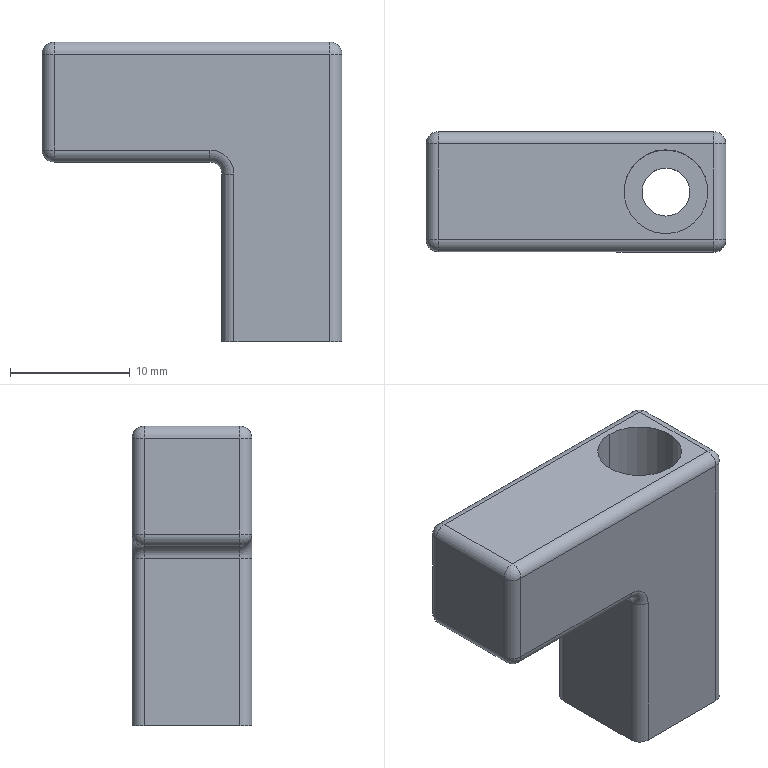NC program | NX | posted with a generic post | part box 25 x 10 x 25 mm
Lines 1608 to 2000 of 2000:
(ZLEVEL_PROFILE_COPY_1 , TOOL : D6R0.5)
N3202 T08 M6
N3204 G54
N3206 G17 G0 G90 X1.039 Y-7.89 S9500 M3
N3208 G43 Z11. H8
N3210 Z1.488
N3212 G94 G1 Z-0.012 F1000.
N3214 X0.52 Y-6.99
N3216 G3 X0. Y-6.69 R0.6
N3218 G1 X-11.5 F3000.
N3220 G2 X-14.19 Y-4. R2.69
N3222 G1 Y4.
N3224 G2 X-11.5 Y6.69 R2.69
N3226 G1 X11.5
N3228 G2 X14.19 Y4. R2.69
N3230 G1 Y-4.
N3232 G2 X11.5 Y-6.69 R2.69
N3234 G1 X0.
N3236 Y-6.751 Z-0.021
N3238 Y-6.8 Z-0.03
N3240 X11.5
N3242 G3 X14.3 Y-4. R2.8
N3244 G1 Y4.
N3246 G3 X11.5 Y6.8 R2.8
N3248 G1 X-11.5
N3250 G3 X-14.3 Y4. R2.8
N3252 G1 Y-4.
N3254 G3 X-11.5 Y-6.8 R2.8
N3256 G1 X0.
N3258 Y-6.856 Z-0.043
N3260 Y-6.903 Z-0.055
N3262 X-11.5
N3264 G2 X-14.403 Y-4. R2.903
N3266 G1 Y4.
N3268 G2 X-11.5 Y6.903 R2.903
N3270 G1 X11.5
N3272 G2 X14.403 Y4. R2.903
N3274 G1 Y-4.
N3276 G2 X11.5 Y-6.903 R2.903
N3278 G1 X0.
N3280 Y-6.955 Z-0.071
N3282 Y-7.002 Z-0.086
N3284 X11.5
N3286 G3 X14.502 Y-4. R3.002
N3288 G1 Y4.
N3290 G3 X11.5 Y7.002 R3.002
N3292 G1 X-11.5
N3294 G3 X-14.502 Y4. R3.002
N3296 G1 Y-4.
N3298 G3 X-11.5 Y-7.002 R3.002
N3300 G1 X0.
N3302 Y-7.052 Z-0.105
N3304 Y-7.097 Z-0.124
N3306 X-11.5
N3308 G2 X-14.597 Y-4. R3.097
N3310 G1 Y4.
N3312 G2 X-11.5 Y7.097 R3.097
N3314 G1 X11.5
N3316 G2 X14.597 Y4. R3.097
N3318 G1 Y-4.
N3320 G2 X11.5 Y-7.097 R3.097
N3322 G1 X0.
N3324 Y-7.145 Z-0.146
N3326 Y-7.189 Z-0.167
N3328 X11.5
N3330 G3 X14.689 Y-4. R3.189
N3332 G1 Y4.
N3334 G3 X11.5 Y7.189 R3.189
N3336 G1 X-11.5
N3338 G3 X-14.689 Y4. R3.189
N3340 G1 Y-4.
N3342 G3 X-11.5 Y-7.189 R3.189
N3344 G1 X0.
N3346 Y-7.234 Z-0.192
N3348 Y-7.277 Z-0.217
N3350 X-11.5
N3352 G2 X-14.777 Y-4. R3.277
N3354 G1 Y4.
N3356 G2 X-11.5 Y7.277 R3.277
N3358 G1 X11.5
N3360 G2 X14.777 Y4. R3.277
N3362 G1 Y-4.
N3364 G2 X11.5 Y-7.277 R3.277
N3366 G1 X0.
N3368 Y-7.321 Z-0.244
N3370 Y-7.361 Z-0.272
N3372 X11.5
N3374 G3 X14.861 Y-4. R3.361
N3376 G1 Y4.
N3378 G3 X11.5 Y7.361 R3.361
N3380 G1 X-11.5
N3382 G3 X-14.861 Y4. R3.361
N3384 G1 Y-4.
N3386 G3 X-11.5 Y-7.361 R3.361
N3388 G1 X0.
N3390 Y-7.403 Z-0.302
N3392 Y-7.442 Z-0.333
N3394 X-11.5
N3396 G2 X-14.942 Y-4. R3.442
N3398 G1 Y4.
N3400 G2 X-11.5 Y7.442 R3.442
N3402 G1 X11.5
N3404 G2 X14.942 Y4. R3.442
N3406 G1 Y-4.
N3408 G2 X11.5 Y-7.442 R3.442
N3410 G1 X0.
N3412 Y-7.481 Z-0.365
N3414 Y-7.518 Z-0.398
N3416 X11.5
N3418 G3 X15.018 Y-4. R3.518
N3420 G1 Y4.
N3422 G3 X11.5 Y7.518 R3.518
N3424 G1 X-11.5
N3426 G3 X-15.018 Y4. R3.518
N3428 G1 Y-4.
N3430 G3 X-11.5 Y-7.518 R3.518
N3432 G1 X0.
N3434 Y-7.555 Z-0.434
N3436 Y-7.589 Z-0.469
N3438 X-11.5
N3440 G2 X-15.089 Y-4. R3.589
N3442 G1 Y4.
N3444 G2 X-11.5 Y7.589 R3.589
N3446 G1 X11.5
N3448 G2 X15.089 Y4. R3.589
N3450 G1 Y-4.
N3452 G2 X11.5 Y-7.589 R3.589
N3454 G1 X0.
N3456 Y-7.624 Z-0.506
N3458 Y-7.656 Z-0.544
N3460 X11.5
N3462 G3 X15.156 Y-4. R3.656
N3464 G1 Y4.
N3466 G3 X11.5 Y7.656 R3.656
N3468 G1 X-11.5
N3470 G3 X-15.156 Y4. R3.656
N3472 G1 Y-4.
N3474 G3 X-11.5 Y-7.656 R3.656
N3476 G1 X0.
N3478 Y-7.688 Z-0.584
N3480 Y-7.717 Z-0.623
N3482 X-11.5
N3484 G2 X-15.217 Y-4. R3.717
N3486 G1 Y4.
N3488 G2 X-11.5 Y7.717 R3.717
N3490 G1 X11.5
N3492 G2 X15.217 Y4. R3.717
N3494 G1 Y-4.
N3496 G2 X11.5 Y-7.717 R3.717
N3498 G1 X0.
N3500 Y-7.746 Z-0.665
N3502 Y-7.773 Z-0.707
N3504 X11.5
N3506 G3 X15.273 Y-4. R3.773
N3508 G1 Y4.
N3510 G3 X11.5 Y7.773 R3.773
N3512 G1 X-11.5
N3514 G3 X-15.273 Y4. R3.773
N3516 G1 Y-4.
N3518 G3 X-11.5 Y-7.773 R3.773
N3520 G1 X0.
N3522 Y-7.799 Z-0.75
N3524 Y-7.823 Z-0.793
N3526 X-11.5
N3528 G2 X-15.323 Y-4. R3.823
N3530 G1 Y4.
N3532 G2 X-11.5 Y7.823 R3.823
N3534 G1 X11.5
N3536 G2 X15.323 Y4. R3.823
N3538 G1 Y-4.
N3540 G2 X11.5 Y-7.823 R3.823
N3542 G1 X0.
N3544 Y-7.846 Z-0.838
N3546 Y-7.867 Z-0.883
N3548 X11.5
N3550 G3 X15.367 Y-4. R3.867
N3552 G1 Y4.
N3554 G3 X11.5 Y7.867 R3.867
N3556 G1 X-11.5
N3558 G3 X-15.367 Y4. R3.867
N3560 G1 Y-4.
N3562 G3 X-11.5 Y-7.867 R3.867
N3564 G1 X0.
N3566 Y-7.887 Z-0.93
N3568 Y-7.905 Z-0.976
N3570 X-11.5
N3572 G2 X-15.405 Y-4. R3.905
N3574 G1 Y4.
N3576 G2 X-11.5 Y7.905 R3.905
N3578 G1 X11.5
N3580 G2 X15.405 Y4. R3.905
N3582 G1 Y-4.
N3584 G2 X11.5 Y-7.905 R3.905
N3586 G1 X0.
N3588 Y-7.922 Z-1.023
N3590 Y-7.937 Z-1.071
N3592 X11.5
N3594 G3 X15.437 Y-4. R3.937
N3596 G1 Y4.
N3598 G3 X11.5 Y7.937 R3.937
N3600 G1 X-11.5
N3602 G3 X-15.437 Y4. R3.937
N3604 G1 Y-4.
N3606 G3 X-11.5 Y-7.937 R3.937
N3608 G1 X0.
N3610 Y-7.951 Z-1.119
N3612 Y-7.963 Z-1.168
N3614 X-11.5
N3616 G2 X-15.463 Y-4. R3.963
N3618 G1 Y4.
N3620 G2 X-11.5 Y7.963 R3.963
N3622 G1 X11.5
N3624 G2 X15.463 Y4. R3.963
N3626 G1 Y-4.
N3628 G2 X11.5 Y-7.963 R3.963
N3630 G1 X0.
N3632 Y-7.972 Z-1.209
N3634 Y-7.979 Z-1.251
N3636 X11.5
N3638 G3 X15.479 Y-4. R3.979
N3640 G1 Y4.
N3642 G3 X11.5 Y7.979 R3.979
N3644 G1 X-11.5
N3646 G3 X-15.479 Y4. R3.979
N3648 G1 Y-4.
N3650 G3 X-11.5 Y-7.979 R3.979
N3652 G1 X0.
N3654 Y-7.986 Z-1.292
N3656 Y-7.991 Z-1.334
N3658 X-11.5
N3660 G2 X-15.491 Y-4. R3.991
N3662 G1 Y4.
N3664 G2 X-11.5 Y7.991 R3.991
N3666 G1 X11.5
N3668 G2 X15.491 Y4. R3.991
N3670 G1 Y-4.
N3672 G2 X11.5 Y-7.991 R3.991
N3674 G1 X0.
N3676 Y-7.998 Z-1.417
N3678 X11.528
N3680 G3 X13.042 Y-7.688 R3.998
N3682 G1 X13.105 Y-7.661
N3684 X13.45 Y-7.49
N3686 G3 X13.662 Y-7.363 R3.998
N3688 G1 X13.958 Y-7.153
N3690 G3 X15.498 Y-4. R3.998
N3692 G1 Y4.
N3694 G3 X11.5 Y7.998 R3.998
N3696 G1 X-11.5
N3698 G3 X-15.448 Y4.626 R3.998
N3700 G1 X-15.487 Y4.283
N3702 X-15.491 Y4.235
N3704 G3 X-15.498 Y4. R3.998
N3706 G1 Y-4.
N3708 G3 X-11.726 Y-7.991 R3.998
N3710 G1 X-11.644 Y-7.995
N3712 X-11.5 Y-7.998
N3714 X0.
N3716 Z-1.5
N3718 X-11.51
N3720 G2 X-15.498 Y-4.01 R3.997
N3722 G1 Y-3.598
N3724 Y3.941
N3726 G2 X-15.448 Y4.626 R3.987
N3728 X-11.51 Y8. R3.996
N3730 G1 X11.5
N3732 G2 X15.499 Y4.01 R4.
N3734 G1 X15.5 Y-3.941
N3736 G2 X13.053 Y-7.683 R3.999
N3738 G1 X12.932 Y-7.732
N3740 G2 X11.528 Y-7.998 R3.95
N3742 G1 X3.449
N3744 Y-7.997
N3746 X3.104
N3748 Y-7.998
N3750 X0.
N3752 G3 X-0.52 Y-8.298 R0.6
N3754 G1 X-1.039 Y-9.198
N3756 Z0.
N3758 G0 Z11.
N3760 M5
(DRILLING_COPY , TOOL : D4A45)
N3762 T02 M6
N3764 G54
N3766 G17 G0 G90 X7.5 Y0. S5000 M3
N3768 G43 Z30. H2
N3770 G94 G81 G98 Z-1. F250. R3.
N3772 G80
N3774 G0 X7.5 Y0. Z30.
N3776 M5
(DRILLING_COPY_COPY_COPY_COPY , TOOL : 4.0ZT)
N3778 T14 M6
N3780 G54
N3782 G17 G0 G90 X7.5 Y0. S1910 M3
N3784 G43 Z30. H14
N3786 G94 G83 G98 Z-27.702 F180. Q2. R3.
N3788 G80
N3790 G0 X7.5 Y0. Z30.
N3792 M5
(HOLE_MILLING , TOOL : D4)
N3794 T04 M6
N3796 G54
N3798 G17 G0 G90 X7.5 Y0. S9500 M3
N3800 G43 Z11. H4
N3802 Z0.5
N3804 G94 G3 X8.25 Y-0.75 R0.75 F1250.
N3806 X9. Y0. R0.75
N3808 X9. Y0. Z0.2 I-1.5 J0.
N3810 X9. Y0. Z-0.1 I-1.5 J0.
N3812 X9. Y0. Z-0.4 I-1.5 J0.
N3814 X9. Y0. Z-0.7 I-1.5 J0.
N3816 X9. Y0. Z-1. I-1.5 J0.
N3818 X9. Y0. Z-1.3 I-1.5 J0.
N3820 X9. Y0. Z-1.6 I-1.5 J0.
N3822 X9. Y0. Z-1.9 I-1.5 J0.
N3824 X9. Y0. Z-2.2 I-1.5 J0.
N3826 X9. Y0. Z-2.5 I-1.5 J0.
N3828 X9. Y0. Z-2.8 I-1.5 J0.
N3830 X9. Y0. Z-3.1 I-1.5 J0.
N3832 X9. Y0. Z-3.4 I-1.5 J0.
N3834 X9. Y0. Z-3.7 I-1.5 J0.
N3836 X9. Y0. Z-4. I-1.5 J0.
N3838 X9. Y0. Z-4.3 I-1.5 J0.
N3840 X9. Y0. Z-4.6 I-1.5 J0.
N3842 X9. Y0. Z-4.9 I-1.5 J0.
N3844 X9. Y0. Z-5.2 I-1.5 J0.
N3846 X9. Y0. Z-5.5 I-1.5 J0.
N3848 X9. Y0. Z-5.8 I-1.5 J0.
N3850 X9. Y0. Z-6.1 I-1.5 J0.
N3852 X9. Y0. Z-6.4 I-1.5 J0.
N3854 X9. Y0. Z-6.7 I-1.5 J0.
N3856 X9. Y0. Z-7. I-1.5 J0.
N3858 X9. Y0. Z-7.3 I-1.5 J0.
N3860 X9. Y0. Z-7.6 I-1.5 J0.
N3862 X9. Y0. Z-7.9 I-1.5 J0.
N3864 X9. Y0. Z-8.2 I-1.5 J0.
N3866 X9. Y0. Z-8.5 I-1.5 J0.
N3868 X9. Y0. Z-8.8 I-1.5 J0.
N3870 X9. Y0. Z-9.1 I-1.5 J0.
N3872 X9. Y0. Z-9.4 I-1.5 J0.
N3874 X9. Y0. Z-9.7 I-1.5 J0.
N3876 X9. Y0. Z-10. I-1.5 J0.
N3878 X9. Y0. Z-10.3 I-1.5 J0.
N3880 X9. Y0. Z-10.6 I-1.5 J0.
N3882 X9. Y0. Z-10.9 I-1.5 J0.
N3884 X9. Y0. Z-11.2 I-1.5 J0.
N3886 X9. Y0. Z-11.5 I-1.5 J0.
N3888 X9. Y0. Z-11.8 I-1.5 J0.
N3890 X9. Y0. Z-12.1 I-1.5 J0.
N3892 X9. Y0. Z-12.4 I-1.5 J0.
N3894 X9. Y0. Z-12.7 I-1.5 J0.
N3896 X9. Y0. Z-13. I-1.5 J0.
N3898 X9. Y0. Z-13.3 I-1.5 J0.
N3900 X9. Y0. Z-13.6 I-1.5 J0.
N3902 X9. Y0. Z-13.9 I-1.5 J0.
N3904 X9. Y0. Z-14.2 I-1.5 J0.
N3906 X9. Y0. Z-14.5 I-1.5 J0.
N3908 X9. Y0. Z-14.8 I-1.5 J0.
N3910 X6.75 Y-1.299 Z-15. R-1.5
N3912 X8.799 Y-0.75 R1.5
N3914 X6.75 Y-1.299 R-1.5
N3916 X7.775 Y-1.025 R0.75
N3918 X7.5 Y0. R0.75
N3920 G0 Z11.
N3922 M5
(ZLEVEL_PROFILE_1_COPY_1_COPY , TOOL : D4A45)
N3924 T02 M6
N3926 G54
N3928 G17 G0 G90 X8.307 Y1.543 S9500 M3
N3930 G43 Z11. H2
N3932 Z0.
N3934 G94 G1 Z-1. F1000.
N3936 X7.846 Y2.341
N3938 G3 X7.5 Y2.541 R0.4
N3940 G1 X7.495
N3942 G3 X4.959 Y-0.005 R2.541
N3944 X7.5 Y2.541 R-2.541
N3946 X7.154 Y2.341 R0.4
N3948 G1 X6.693 Y1.543
N3950 Z0.
N3952 G0 Z11.
N3954 M5
N3956 M2